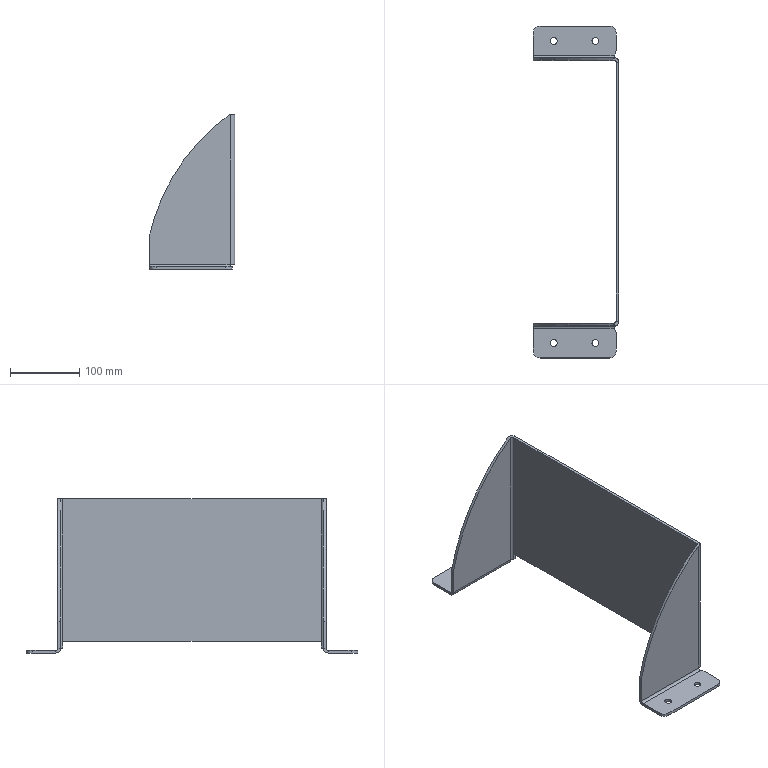Part | STEP file | ZSYP1V11 | 1 solid | 58 faces | box 124 x 480 x 223 mm | volume 511091 mm3 | plane 34 | cylinder 22 | spline 2 | commonest cylinder face diameters 10 x8 6 x4 14 x4 20 x4 594.956 x2